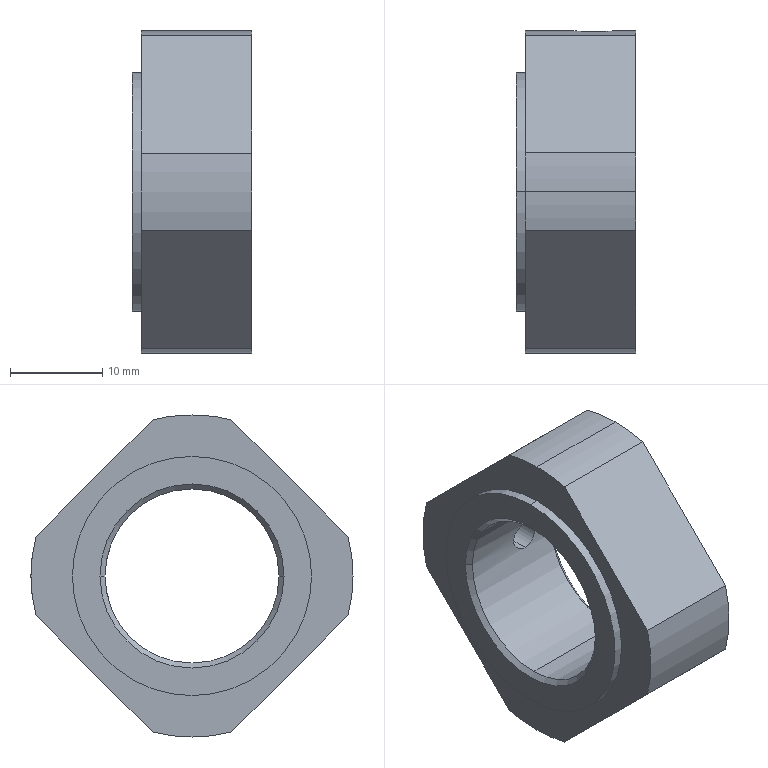Part | STEP file | 0244_Z_002_BSW20_3 | 1 solid | 24 faces | box 13 x 35 x 35 mm | volume 6873 mm3 | cylinder 11 | plane 7 | cone 6 | commonest cylinder face diameters 35 x5 3.242 x2 18.917 x2 26 x2